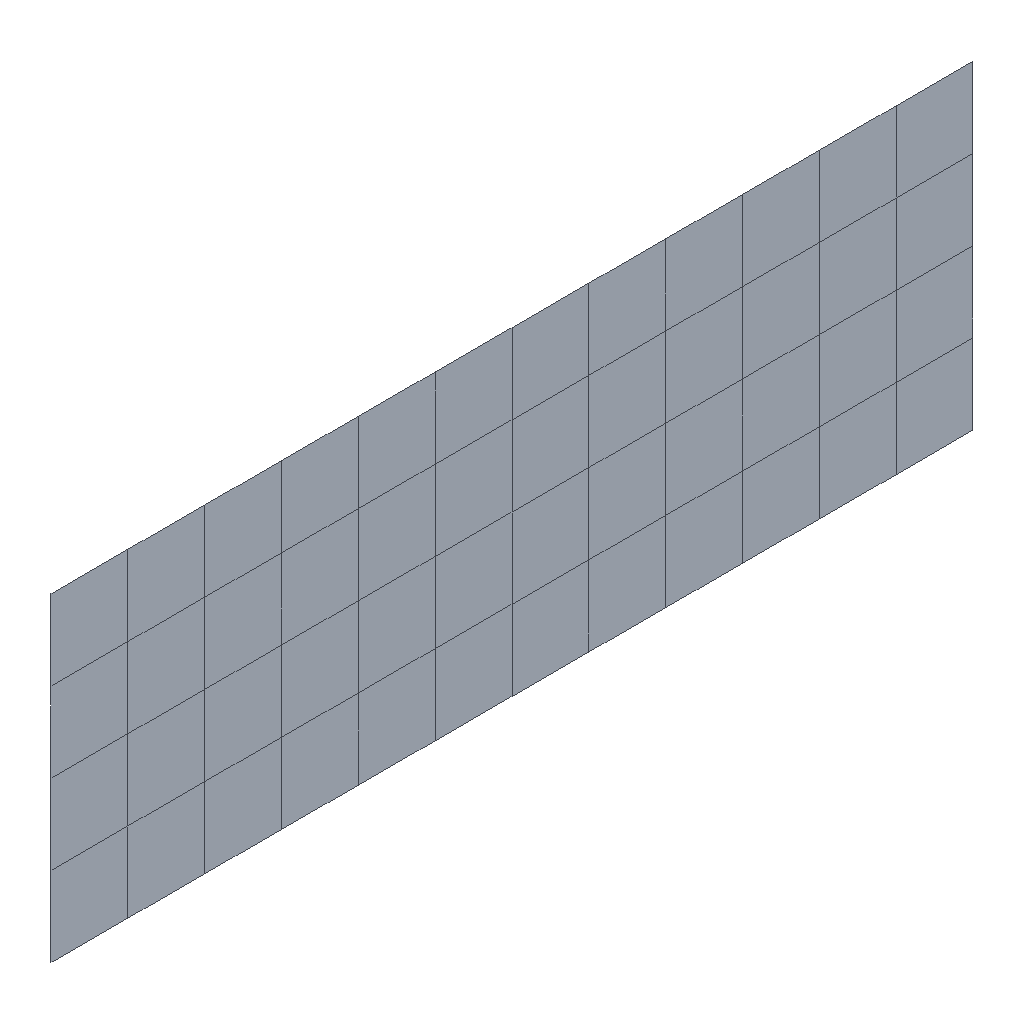Simulation study | abaqus
Set-up summary:
category,name,step,type,value,unit,region
solver,abaqus,,Abaqus/CAE 2024
units,SI m-kg-s (Pa),,inferred,E=3e+10 density=
analysis,Apply pressure,,static,nlgeom=True; time_period=1
mesh,nodes,,,177
mesh,elements,,,48
element_type,S8R5,,,48
material,Metal,,E,3e+10
material,Metal,,nu,0.3
load,Pressure,Apply pressure,pressure,20000,,_G7
bc,Fix,Apply pressure,encastre,[dofs=ENCASTRE],,EndA
bc,Rail,Apply pressure,fixed,"[dofs=rx,ry,rz,y,z n=5]",,EndB
Abaqus input file, long lists of numbers shortened:
*Heading
** Job name: deck Model name: Model-1
** Generated by: Abaqus/CAE 2024
*Preprint, echo=NO, model=NO, history=NO, contact=NO
**
** PARTS
**
*Part, name=Plate
*Node
      1,         -0.5, 0.08868,           0.
      2,         -0.5,  0.4887,           0.
** (175 more lines like these left out)
*Element, type=S8R5
 1,   1,   7,  36,  22,  66,  67,  68,  69
 2,   7,   8,  37,  36,  70,  71,  72,  67
** (46 more lines like these left out)
*Nset, nset=_G4, internal, generate
   1,  177,    1
*Elset, elset=_G4, internal, generate
  1,  48,   1
*Orientation, name=Ori-1
-0.866,         -0.5,           0.,         -0.5, 0.866,           0.
3, 0.
** Section: PlateSection
*Shell General Section, elset=_G4, material=Metal, orientation=Ori-1
0.008,
*End Part
**
**
** ASSEMBLY
**
*Assembly, name=Assembly
**
*Instance, name=Plate-1, part=Plate
*End Instance
**
*Nset, nset=EndA, instance=Plate-1
   3,   4,  15,  16,  17, 116, 119, 121, 123
*Elset, elset=EndA, instance=Plate-1, generate
 21,  24,   1
*Nset, nset=EndB, instance=Plate-1
   5,   6,  28,  29,  30, 170, 173, 175, 177
*Elset, elset=EndB, instance=Plate-1, generate
 45,  48,   1
*Nset, nset=MidSpan, instance=Plate-1
  1,  2,  7,  8,  9, 66, 70, 73, 76
*Elset, elset=MidSpan, instance=Plate-1
  1,  2,  3,  4, 25, 26, 27, 28
*Elset, elset=__G7_SPOS, internal, instance=Plate-1, generate
  1,  48,   1
*Surface, type=ELEMENT, name=_G7, internal
__G7_SPOS, SPOS
*Nset, nset="_T-Plate-1-Datum csys-1", internal
EndB,
*Transform, nset="_T-Plate-1-Datum csys-1"
-0.866,         -0.5,           0.,         -0.5, 0.866,           0.
*End Assembly
**
** MATERIALS
**
*Material, name=Metal
*Elastic
 3e+10, 0.3
** ----------------------------------------------------------------
**
** STEP: Apply pressure
**
*Step, name="Apply pressure", nlgeom=YES
Nonlinear analysis: Uniform pressure (20 kPa) load
*Static
0.1, 1., 1e-05, 1.
**
** BOUNDARY CONDITIONS
**
** Name: Fix left end Type: Symmetry/Antisymmetry/Encastre
*Boundary
EndA, ENCASTRE
** Name: Rail boundary condition Type: Displacement/Rotation
*Boundary
EndB, 2, 2
EndB, 3, 3
EndB, 4, 4
EndB, 5, 5
EndB, 6, 6
**
** LOADS
**
** Name: Pressure   Type: Pressure
*Dsload
_G7, P, 20000.
**
** OUTPUT REQUESTS
**
*Restart, write, frequency=0
**
** FIELD OUTPUT: F-Output-1
**
*Output, field, variable=PRESELECT, frequency=2
**
** HISTORY OUTPUT: H-Output-1
**
*Output, history
*Node Output, nset=MidSpan
U3,
*End Step
Results summary:
result,odb.job_status,,,JOB_STATUS_COMPLETED_SUCCESSFULLY,"consistent, unstated (Abaqus has no unit system)"
result,steps[0].procedure,Apply pressure,,*STATIC,"consistent, unstated (Abaqus has no unit system)"
result,steps[0].time_period,Apply pressure,,1,"consistent, unstated (Abaqus has no unit system)"
result,steps[0].n_frames,Apply pressure,,4,"consistent, unstated (Abaqus has no unit system)"
result,steps[0].last_frame.id,Apply pressure,,6,"consistent, unstated (Abaqus has no unit system)"
result,steps[0].last_frame.value,Apply pressure,,1,"consistent, unstated (Abaqus has no unit system)"
result,steps[0].last_frame.description,Apply pressure,,Increment      6: Step Time =    1.000,"consistent, unstated (Abaqus has no unit system)"
result,steps[0].completed,Apply pressure,,True,"consistent, unstated (Abaqus has no unit system)"
result,steps[0].max_U_magnitude,Apply pressure,,0.05087,"consistent, unstated (Abaqus has no unit system)"
result,steps[0].max_S_mises,Apply pressure,,2.41886e+08,"consistent, unstated (Abaqus has no unit system)"
result,steps[0].RF_sum[1],Apply pressure,,23.657,"consistent, unstated (Abaqus has no unit system)"
result,steps[0].RF_sum[2],Apply pressure,,-40.789,"consistent, unstated (Abaqus has no unit system)"
result,steps[0].RF_sum[3],Apply pressure,,7963.14,"consistent, unstated (Abaqus has no unit system)"